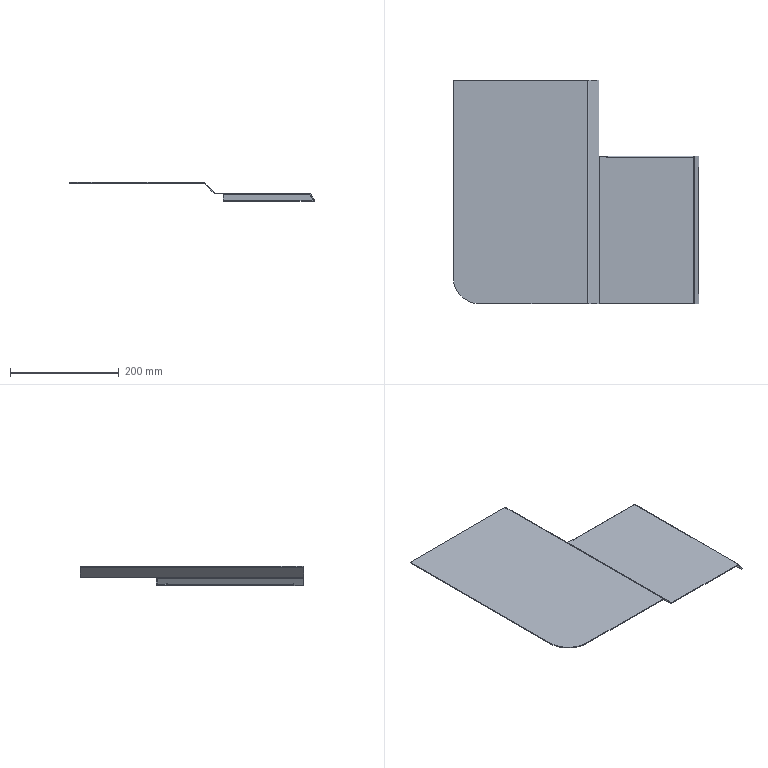Part | SolidWorks | features MirrorStock 1 | 1 solid | 72 faces | box 452.1 x 411.5 x 35.646 mm | volume 260471 mm3 | plane 54 | cylinder 17 | spline 1 | commonest cylinder face diameters 4 x6 1 x4 6.4 x4 7 x2 97.4 x1